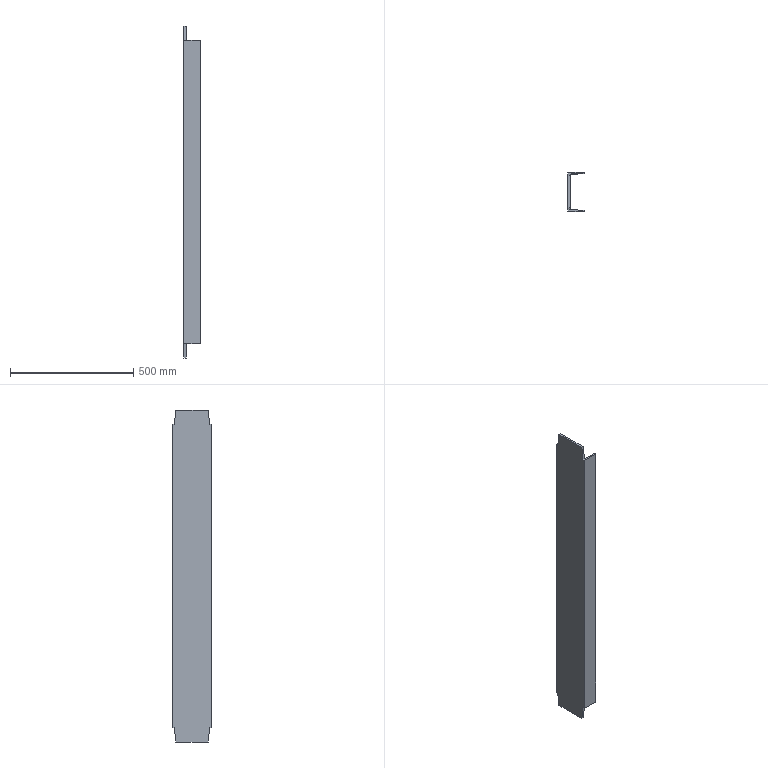Part | SolidWorks | features Extrusion 1, ICE 1 | 1 solid | 18 faces | box 65 x 160 x 1348 mm | volume 2648614 mm3 | plane 18
STEP:
#1=CARTESIAN_POINT('',(0.,146.,-674.));
#2=VERTEX_POINT('',#1);
#3=CARTESIAN_POINT('',(0.,14.,-674.));
#4=VERTEX_POINT('',#3);
#5=CARTESIAN_POINT('',(0.,0.,-674.));
#6=DIRECTION('',(0.,-1.,0.));
#7=VECTOR('',#6,1000.);
#8=LINE('',#5,#7);
#9=EDGE_CURVE('',#2,#4,#8,.T.);
#10=ORIENTED_EDGE('',*,*,#9,.T.);
#11=CARTESIAN_POINT('',(0.,8.,-617.));
#12=VERTEX_POINT('',#11);
#13=CARTESIAN_POINT('',(0.,8.,-617.));
#14=DIRECTION('',(0.,0.1047,-0.9945));
#15=VECTOR('',#14,1000.);
#16=LINE('',#13,#15);
#17=EDGE_CURVE('',#12,#4,#16,.T.);
#18=ORIENTED_EDGE('',*,*,#17,.F.);
#19=CARTESIAN_POINT('',(0.,0.,-617.));
#20=VERTEX_POINT('',#19);
#21=CARTESIAN_POINT('',(0.,0.,-617.));
#22=DIRECTION('',(0.,1.,0.));
#23=VECTOR('',#22,1000.);
#24=LINE('',#21,#23);
#25=EDGE_CURVE('',#20,#12,#24,.T.);
#26=ORIENTED_EDGE('',*,*,#25,.F.);
#27=CARTESIAN_POINT('',(0.,0.,617.));
#28=VERTEX_POINT('',#27);
#29=CARTESIAN_POINT('',(0.,0.,674.));
#30=DIRECTION('',(0.,0.,-1.));
#31=VECTOR('',#30,1000.);
#32=LINE('',#29,#31);
#33=EDGE_CURVE('',#28,#20,#32,.T.);
#34=ORIENTED_EDGE('',*,*,#33,.F.);
#35=CARTESIAN_POINT('',(0.,8.,617.));
#36=VERTEX_POINT('',#35);
#37=CARTESIAN_POINT('',(0.,0.,617.));
#38=DIRECTION('',(0.,-1.,0.));
#39=VECTOR('',#38,1000.);
#40=LINE('',#37,#39);
#41=EDGE_CURVE('',#36,#28,#40,.T.);
#42=ORIENTED_EDGE('',*,*,#41,.F.);
#43=CARTESIAN_POINT('',(0.,14.,674.));
#44=VERTEX_POINT('',#43);
#45=CARTESIAN_POINT('',(0.,8.,617.));
#46=DIRECTION('',(0.,-0.1047,-0.9945));
#47=VECTOR('',#46,1000.);
#48=LINE('',#45,#47);
#49=EDGE_CURVE('',#44,#36,#48,.T.);
#50=ORIENTED_EDGE('',*,*,#49,.F.);
#51=CARTESIAN_POINT('',(0.,146.,674.));
#52=VERTEX_POINT('',#51);
#53=CARTESIAN_POINT('',(0.,0.,674.));
#54=DIRECTION('',(0.,-1.,0.));
#55=VECTOR('',#54,1000.);
#56=LINE('',#53,#55);
#57=EDGE_CURVE('',#52,#44,#56,.T.);
#58=ORIENTED_EDGE('',*,*,#57,.F.);
#59=CARTESIAN_POINT('',(0.,152.,617.));
#60=VERTEX_POINT('',#59);
#61=CARTESIAN_POINT('',(0.,152.,617.));
#62=DIRECTION('',(0.,-0.1047,0.9945));
#63=VECTOR('',#62,1000.);
#64=LINE('',#61,#63);
#65=EDGE_CURVE('',#60,#52,#64,.T.);
#66=ORIENTED_EDGE('',*,*,#65,.F.);
#67=CARTESIAN_POINT('',(0.,160.,617.));
#68=VERTEX_POINT('',#67);
#69=CARTESIAN_POINT('',(0.,160.,617.));
#70=DIRECTION('',(0.,-1.,0.));
#71=VECTOR('',#70,1000.);
#72=LINE('',#69,#71);
#73=EDGE_CURVE('',#68,#60,#72,.T.);
#74=ORIENTED_EDGE('',*,*,#73,.F.);
#75=CARTESIAN_POINT('',(0.,160.,-617.));
#76=VERTEX_POINT('',#75);
#77=CARTESIAN_POINT('',(0.,160.,674.));
#78=DIRECTION('',(0.,0.,-1.));
#79=VECTOR('',#78,1000.);
#80=LINE('',#77,#79);
#81=EDGE_CURVE('',#68,#76,#80,.T.);
#82=ORIENTED_EDGE('',*,*,#81,.T.);
#83=CARTESIAN_POINT('',(0.,152.,-617.));
#84=VERTEX_POINT('',#83);
#85=CARTESIAN_POINT('',(0.,160.,-617.));
#86=DIRECTION('',(0.,1.,0.));
#87=VECTOR('',#86,1000.);
#88=LINE('',#85,#87);
#89=EDGE_CURVE('',#84,#76,#88,.T.);
#90=ORIENTED_EDGE('',*,*,#89,.F.);
#91=CARTESIAN_POINT('',(0.,152.,-617.));
#92=DIRECTION('',(0.,0.1047,0.9945));
#93=VECTOR('',#92,1000.);
#94=LINE('',#91,#93);
#95=EDGE_CURVE('',#2,#84,#94,.T.);
#96=ORIENTED_EDGE('',*,*,#95,.F.);
#97=EDGE_LOOP('',(#10,#18,#26,#34,#42,#50,#58,#66,#74,#82,#90,#96));
#98=FACE_OUTER_BOUND('',#97,.T.);
#99=CARTESIAN_POINT('',(0.,0.,674.));
#100=DIRECTION('',(1.,0.,0.));
#101=DIRECTION('',(0.,0.,-1.));
#102=AXIS2_PLACEMENT_3D('',#99,#100,#101);
#103=PLANE('',#102);
#104=ADVANCED_FACE('',(#98),#103,.F.);
#105=ORIENTED_EDGE('',*,*,#33,.T.);
#106=CARTESIAN_POINT('',(65.,0.,-617.));
#107=VERTEX_POINT('',#106);
#108=CARTESIAN_POINT('',(65.,0.,-617.));
#109=DIRECTION('',(-1.,0.,0.));
#110=VECTOR('',#109,1000.);
#111=LINE('',#108,#110);
#112=EDGE_CURVE('',#107,#20,#111,.T.);
#113=ORIENTED_EDGE('',*,*,#112,.F.);
#114=CARTESIAN_POINT('',(65.,0.,617.));
#115=VERTEX_POINT('',#114);
#116=CARTESIAN_POINT('',(65.,0.,674.));
#117=DIRECTION('',(0.,0.,-1.));
#118=VECTOR('',#117,1000.);
#119=LINE('',#116,#118);
#120=EDGE_CURVE('',#115,#107,#119,.T.);
#121=ORIENTED_EDGE('',*,*,#120,.F.);
#122=CARTESIAN_POINT('',(65.,0.,617.));
#123=DIRECTION('',(-1.,0.,0.));
#124=VECTOR('',#123,1000.);
#125=LINE('',#122,#124);
#126=EDGE_CURVE('',#115,#28,#125,.T.);
#127=ORIENTED_EDGE('',*,*,#126,.T.);
#128=EDGE_LOOP('',(#105,#113,#121,#127));
#129=FACE_OUTER_BOUND('',#128,.T.);
#130=CARTESIAN_POINT('',(0.,0.,674.));
#131=DIRECTION('',(0.,1.,0.));
#132=DIRECTION('',(0.,0.,1.));
#133=AXIS2_PLACEMENT_3D('',#130,#131,#132);
#134=PLANE('',#133);
#135=ADVANCED_FACE('',(#129),#134,.F.);
#136=ORIENTED_EDGE('',*,*,#120,.T.);
#137=CARTESIAN_POINT('',(65.,4.,-617.));
#138=VERTEX_POINT('',#137);
#139=CARTESIAN_POINT('',(65.,0.,-617.));
#140=DIRECTION('',(0.,1.,0.));
#141=VECTOR('',#140,1000.);
#142=LINE('',#139,#141);
#143=EDGE_CURVE('',#107,#138,#142,.T.);
#144=ORIENTED_EDGE('',*,*,#143,.T.);
#145=CARTESIAN_POINT('',(65.,4.,617.));
#146=VERTEX_POINT('',#145);
#147=CARTESIAN_POINT('',(65.,4.,674.));
#148=DIRECTION('',(0.,0.,-1.));
#149=VECTOR('',#148,1000.);
#150=LINE('',#147,#149);
#151=EDGE_CURVE('',#146,#138,#150,.T.);
#152=ORIENTED_EDGE('',*,*,#151,.F.);
#153=CARTESIAN_POINT('',(65.,0.,617.));
#154=DIRECTION('',(0.,-1.,0.));
#155=VECTOR('',#154,1000.);
#156=LINE('',#153,#155);
#157=EDGE_CURVE('',#146,#115,#156,.T.);
#158=ORIENTED_EDGE('',*,*,#157,.T.);
#159=EDGE_LOOP('',(#136,#144,#152,#158));
#160=FACE_OUTER_BOUND('',#159,.T.);
#161=CARTESIAN_POINT('',(65.,0.,674.));
#162=DIRECTION('',(-1.,0.,0.));
#163=DIRECTION('',(0.,0.,1.));
#164=AXIS2_PLACEMENT_3D('',#161,#162,#163);
#165=PLANE('',#164);
#166=ADVANCED_FACE('',(#160),#165,.F.);
#167=ORIENTED_EDGE('',*,*,#151,.T.);
#168=CARTESIAN_POINT('',(8.5,8.,-617.));
#169=VERTEX_POINT('',#168);
#170=CARTESIAN_POINT('',(65.,4.,-617.));
#171=DIRECTION('',(-0.9975,0.07062,0.));
#172=VECTOR('',#171,1000.);
#173=LINE('',#170,#172);
#174=EDGE_CURVE('',#138,#169,#173,.T.);
#175=ORIENTED_EDGE('',*,*,#174,.T.);
#176=CARTESIAN_POINT('',(8.5,8.,617.));
#177=VERTEX_POINT('',#176);
#178=CARTESIAN_POINT('',(8.5,8.,674.));
#179=DIRECTION('',(0.,0.,-1.));
#180=VECTOR('',#179,1000.);
#181=LINE('',#178,#180);
#182=EDGE_CURVE('',#177,#169,#181,.T.);
#183=ORIENTED_EDGE('',*,*,#182,.F.);
#184=CARTESIAN_POINT('',(65.,4.,617.));
#185=DIRECTION('',(0.9975,-0.07062,0.));
#186=VECTOR('',#185,1000.);
#187=LINE('',#184,#186);
#188=EDGE_CURVE('',#177,#146,#187,.T.);
#189=ORIENTED_EDGE('',*,*,#188,.T.);
#190=EDGE_LOOP('',(#167,#175,#183,#189));
#191=FACE_OUTER_BOUND('',#190,.T.);
#192=CARTESIAN_POINT('',(65.,4.,674.));
#193=DIRECTION('',(-0.07062,-0.9975,0.));
#194=DIRECTION('',(0.9975,-0.07062,0.));
#195=AXIS2_PLACEMENT_3D('',#192,#193,#194);
#196=PLANE('',#195);
#197=ADVANCED_FACE('',(#191),#196,.F.);
#198=ORIENTED_EDGE('',*,*,#182,.T.);
#199=CARTESIAN_POINT('',(8.5,14.,-674.));
#200=VERTEX_POINT('',#199);
#201=CARTESIAN_POINT('',(8.5,-126.405,659.852));
#202=DIRECTION('',(0.,0.1047,-0.9945));
#203=VECTOR('',#202,1000.);
#204=LINE('',#201,#203);
#205=EDGE_CURVE('',#169,#200,#204,.T.);
#206=ORIENTED_EDGE('',*,*,#205,.T.);
#207=CARTESIAN_POINT('',(8.5,146.,-674.));
#208=VERTEX_POINT('',#207);
#209=CARTESIAN_POINT('',(8.5,8.,-674.));
#210=DIRECTION('',(0.,1.,0.));
#211=VECTOR('',#210,1000.);
#212=LINE('',#209,#211);
#213=EDGE_CURVE('',#200,#208,#212,.T.);
#214=ORIENTED_EDGE('',*,*,#213,.T.);
#215=CARTESIAN_POINT('',(8.5,152.,-617.));
#216=VERTEX_POINT('',#215);
#217=CARTESIAN_POINT('',(8.5,284.827,644.86));
#218=DIRECTION('',(0.,0.1047,0.9945));
#219=VECTOR('',#218,1000.);
#220=LINE('',#217,#219);
#221=EDGE_CURVE('',#208,#216,#220,.T.);
#222=ORIENTED_EDGE('',*,*,#221,.T.);
#223=CARTESIAN_POINT('',(8.5,152.,617.));
#224=VERTEX_POINT('',#223);
#225=CARTESIAN_POINT('',(8.5,152.,674.));
#226=DIRECTION('',(0.,0.,-1.));
#227=VECTOR('',#226,1000.);
#228=LINE('',#225,#227);
#229=EDGE_CURVE('',#224,#216,#228,.T.);
#230=ORIENTED_EDGE('',*,*,#229,.F.);
#231=CARTESIAN_POINT('',(8.5,146.,674.));
#232=VERTEX_POINT('',#231);
#233=CARTESIAN_POINT('',(8.5,144.488,688.367));
#234=DIRECTION('',(0.,-0.1047,0.9945));
#235=VECTOR('',#234,1000.);
#236=LINE('',#233,#235);
#237=EDGE_CURVE('',#224,#232,#236,.T.);
#238=ORIENTED_EDGE('',*,*,#237,.T.);
#239=CARTESIAN_POINT('',(8.5,14.,674.));
#240=VERTEX_POINT('',#239);
#241=CARTESIAN_POINT('',(8.5,8.,674.));
#242=DIRECTION('',(0.,1.,0.));
#243=VECTOR('',#242,1000.);
#244=LINE('',#241,#243);
#245=EDGE_CURVE('',#240,#232,#244,.T.);
#246=ORIENTED_EDGE('',*,*,#245,.F.);
#247=CARTESIAN_POINT('',(8.5,13.934,673.375));
#248=DIRECTION('',(0.,-0.1047,-0.9945));
#249=VECTOR('',#248,1000.);
#250=LINE('',#247,#249);
#251=EDGE_CURVE('',#240,#177,#250,.T.);
#252=ORIENTED_EDGE('',*,*,#251,.T.);
#253=EDGE_LOOP('',(#198,#206,#214,#222,#230,#238,#246,#252));
#254=FACE_OUTER_BOUND('',#253,.T.);
#255=CARTESIAN_POINT('',(8.5,8.,674.));
#256=DIRECTION('',(-1.,0.,0.));
#257=DIRECTION('',(0.,0.,1.));
#258=AXIS2_PLACEMENT_3D('',#255,#256,#257);
#259=PLANE('',#258);
#260=ADVANCED_FACE('',(#254),#259,.F.);
#261=CARTESIAN_POINT('',(65.,156.,617.));
#262=VERTEX_POINT('',#261);
#263=CARTESIAN_POINT('',(65.,156.,-617.));
#264=VERTEX_POINT('',#263);
#265=CARTESIAN_POINT('',(65.,156.,674.));
#266=DIRECTION('',(0.,0.,-1.));
#267=VECTOR('',#266,1000.);
#268=LINE('',#265,#267);
#269=EDGE_CURVE('',#262,#264,#268,.T.);
#270=ORIENTED_EDGE('',*,*,#269,.F.);
#271=CARTESIAN_POINT('',(65.,156.,617.));
#272=DIRECTION('',(-0.9975,-0.07062,0.));
#273=VECTOR('',#272,1000.);
#274=LINE('',#271,#273);
#275=EDGE_CURVE('',#262,#224,#274,.T.);
#276=ORIENTED_EDGE('',*,*,#275,.T.);
#277=ORIENTED_EDGE('',*,*,#229,.T.);
#278=CARTESIAN_POINT('',(65.,156.,-617.));
#279=DIRECTION('',(0.9975,0.07062,0.));
#280=VECTOR('',#279,1000.);
#281=LINE('',#278,#280);
#282=EDGE_CURVE('',#216,#264,#281,.T.);
#283=ORIENTED_EDGE('',*,*,#282,.T.);
#284=EDGE_LOOP('',(#270,#276,#277,#283));
#285=FACE_OUTER_BOUND('',#284,.T.);
#286=CARTESIAN_POINT('',(65.,156.,674.));
#287=DIRECTION('',(-0.07062,0.9975,0.));
#288=DIRECTION('',(-0.9975,-0.07062,0.));
#289=AXIS2_PLACEMENT_3D('',#286,#287,#288);
#290=PLANE('',#289);
#291=ADVANCED_FACE('',(#285),#290,.F.);
#292=CARTESIAN_POINT('',(65.,160.,617.));
#293=VERTEX_POINT('',#292);
#294=CARTESIAN_POINT('',(65.,160.,-617.));
#295=VERTEX_POINT('',#294);
#296=CARTESIAN_POINT('',(65.,160.,674.));
#297=DIRECTION('',(0.,0.,-1.));
#298=VECTOR('',#297,1000.);
#299=LINE('',#296,#298);
#300=EDGE_CURVE('',#293,#295,#299,.T.);
#301=ORIENTED_EDGE('',*,*,#300,.F.);
#302=CARTESIAN_POINT('',(65.,160.,617.));
#303=DIRECTION('',(0.,-1.,0.));
#304=VECTOR('',#303,1000.);
#305=LINE('',#302,#304);
#306=EDGE_CURVE('',#293,#262,#305,.T.);
#307=ORIENTED_EDGE('',*,*,#306,.T.);
#308=ORIENTED_EDGE('',*,*,#269,.T.);
#309=CARTESIAN_POINT('',(65.,160.,-617.));
#310=DIRECTION('',(0.,1.,0.));
#311=VECTOR('',#310,1000.);
#312=LINE('',#309,#311);
#313=EDGE_CURVE('',#264,#295,#312,.T.);
#314=ORIENTED_EDGE('',*,*,#313,.T.);
#315=EDGE_LOOP('',(#301,#307,#308,#314));
#316=FACE_OUTER_BOUND('',#315,.T.);
#317=CARTESIAN_POINT('',(65.,160.,674.));
#318=DIRECTION('',(-1.,0.,0.));
#319=DIRECTION('',(0.,0.,1.));
#320=AXIS2_PLACEMENT_3D('',#317,#318,#319);
#321=PLANE('',#320);
#322=ADVANCED_FACE('',(#316),#321,.F.);
#323=ORIENTED_EDGE('',*,*,#81,.F.);
#324=CARTESIAN_POINT('',(65.,160.,617.));
#325=DIRECTION('',(-1.,0.,0.));
#326=VECTOR('',#325,1000.);
#327=LINE('',#324,#326);
#328=EDGE_CURVE('',#293,#68,#327,.T.);
#329=ORIENTED_EDGE('',*,*,#328,.F.);
#330=ORIENTED_EDGE('',*,*,#300,.T.);
#331=CARTESIAN_POINT('',(65.,160.,-617.));
#332=DIRECTION('',(-1.,0.,0.));
#333=VECTOR('',#332,1000.);
#334=LINE('',#331,#333);
#335=EDGE_CURVE('',#295,#76,#334,.T.);
#336=ORIENTED_EDGE('',*,*,#335,.T.);
#337=EDGE_LOOP('',(#323,#329,#330,#336));
#338=FACE_OUTER_BOUND('',#337,.T.);
#339=CARTESIAN_POINT('',(0.,160.,674.));
#340=DIRECTION('',(0.,-1.,0.));
#341=DIRECTION('',(1.,0.,0.));
#342=AXIS2_PLACEMENT_3D('',#339,#340,#341);
#343=PLANE('',#342);
#344=ADVANCED_FACE('',(#338),#343,.F.);
#345=ORIENTED_EDGE('',*,*,#57,.T.);
#346=CARTESIAN_POINT('',(0.,14.,674.));
#347=DIRECTION('',(1.,0.,0.));
#348=VECTOR('',#347,1000.);
#349=LINE('',#346,#348);
#350=EDGE_CURVE('',#44,#240,#349,.T.);
#351=ORIENTED_EDGE('',*,*,#350,.T.);
#352=ORIENTED_EDGE('',*,*,#245,.T.);
#353=CARTESIAN_POINT('',(0.,146.,674.));
#354=DIRECTION('',(-1.,0.,0.));
#355=VECTOR('',#354,1000.);
#356=LINE('',#353,#355);
#357=EDGE_CURVE('',#232,#52,#356,.T.);
#358=ORIENTED_EDGE('',*,*,#357,.T.);
#359=EDGE_LOOP('',(#345,#351,#352,#358));
#360=FACE_OUTER_BOUND('',#359,.T.);
#361=CARTESIAN_POINT('',(0.,0.,674.));
#362=DIRECTION('',(0.,0.,-1.));
#363=DIRECTION('',(-1.,0.,0.));
#364=AXIS2_PLACEMENT_3D('',#361,#362,#363);
#365=PLANE('',#364);
#366=ADVANCED_FACE('',(#360),#365,.F.);
#367=CARTESIAN_POINT('',(0.,14.,-674.));
#368=DIRECTION('',(1.,0.,0.));
#369=VECTOR('',#368,1000.);
#370=LINE('',#367,#369);
#371=EDGE_CURVE('',#4,#200,#370,.T.);
#372=ORIENTED_EDGE('',*,*,#371,.F.);
#373=ORIENTED_EDGE('',*,*,#9,.F.);
#374=CARTESIAN_POINT('',(0.,146.,-674.));
#375=DIRECTION('',(-1.,0.,0.));
#376=VECTOR('',#375,1000.);
#377=LINE('',#374,#376);
#378=EDGE_CURVE('',#208,#2,#377,.T.);
#379=ORIENTED_EDGE('',*,*,#378,.F.);
#380=ORIENTED_EDGE('',*,*,#213,.F.);
#381=EDGE_LOOP('',(#372,#373,#379,#380));
#382=FACE_OUTER_BOUND('',#381,.T.);
#383=CARTESIAN_POINT('',(0.,0.,-674.));
#384=DIRECTION('',(0.,0.,-1.));
#385=DIRECTION('',(-1.,0.,0.));
#386=AXIS2_PLACEMENT_3D('',#383,#384,#385);
#387=PLANE('',#386);
#388=ADVANCED_FACE('',(#382),#387,.T.);
#389=CARTESIAN_POINT('',(65.,152.,-617.));
#390=DIRECTION('',(-1.,0.,0.));
#391=VECTOR('',#390,1000.);
#392=LINE('',#389,#391);
#393=EDGE_CURVE('',#216,#84,#392,.T.);
#394=ORIENTED_EDGE('',*,*,#393,.T.);
#395=ORIENTED_EDGE('',*,*,#89,.T.);
#396=ORIENTED_EDGE('',*,*,#335,.F.);
#397=ORIENTED_EDGE('',*,*,#313,.F.);
#398=ORIENTED_EDGE('',*,*,#282,.F.);
#399=EDGE_LOOP('',(#394,#395,#396,#397,#398));
#400=FACE_OUTER_BOUND('',#399,.T.);
#401=CARTESIAN_POINT('',(65.,160.,-617.));
#402=DIRECTION('',(0.,0.,1.));
#403=DIRECTION('',(0.,-1.,0.));
#404=AXIS2_PLACEMENT_3D('',#401,#402,#403);
#405=PLANE('',#404);
#406=ADVANCED_FACE('',(#400),#405,.F.);
#407=ORIENTED_EDGE('',*,*,#378,.T.);
#408=ORIENTED_EDGE('',*,*,#95,.T.);
#409=ORIENTED_EDGE('',*,*,#393,.F.);
#410=ORIENTED_EDGE('',*,*,#221,.F.);
#411=EDGE_LOOP('',(#407,#408,#409,#410));
#412=FACE_OUTER_BOUND('',#411,.T.);
#413=CARTESIAN_POINT('',(65.,152.,-617.));
#414=DIRECTION('',(0.,-0.9945,0.1047));
#415=DIRECTION('',(0.,-0.1047,-0.9945));
#416=AXIS2_PLACEMENT_3D('',#413,#414,#415);
#417=PLANE('',#416);
#418=ADVANCED_FACE('',(#412),#417,.F.);
#419=ORIENTED_EDGE('',*,*,#143,.F.);
#420=ORIENTED_EDGE('',*,*,#112,.T.);
#421=ORIENTED_EDGE('',*,*,#25,.T.);
#422=CARTESIAN_POINT('',(65.,8.,-617.));
#423=DIRECTION('',(-1.,0.,0.));
#424=VECTOR('',#423,1000.);
#425=LINE('',#422,#424);
#426=EDGE_CURVE('',#169,#12,#425,.T.);
#427=ORIENTED_EDGE('',*,*,#426,.F.);
#428=ORIENTED_EDGE('',*,*,#174,.F.);
#429=EDGE_LOOP('',(#419,#420,#421,#427,#428));
#430=FACE_OUTER_BOUND('',#429,.T.);
#431=CARTESIAN_POINT('',(65.,0.,-617.));
#432=DIRECTION('',(0.,0.,1.));
#433=DIRECTION('',(0.,-1.,0.));
#434=AXIS2_PLACEMENT_3D('',#431,#432,#433);
#435=PLANE('',#434);
#436=ADVANCED_FACE('',(#430),#435,.F.);
#437=ORIENTED_EDGE('',*,*,#426,.T.);
#438=ORIENTED_EDGE('',*,*,#17,.T.);
#439=ORIENTED_EDGE('',*,*,#371,.T.);
#440=ORIENTED_EDGE('',*,*,#205,.F.);
#441=EDGE_LOOP('',(#437,#438,#439,#440));
#442=FACE_OUTER_BOUND('',#441,.T.);
#443=CARTESIAN_POINT('',(65.,8.,-617.));
#444=DIRECTION('',(0.,0.9945,0.1047));
#445=DIRECTION('',(0.,-0.1047,0.9945));
#446=AXIS2_PLACEMENT_3D('',#443,#444,#445);
#447=PLANE('',#446);
#448=ADVANCED_FACE('',(#442),#447,.F.);
#449=ORIENTED_EDGE('',*,*,#306,.F.);
#450=ORIENTED_EDGE('',*,*,#328,.T.);
#451=ORIENTED_EDGE('',*,*,#73,.T.);
#452=CARTESIAN_POINT('',(65.,152.,617.));
#453=DIRECTION('',(-1.,0.,0.));
#454=VECTOR('',#453,1000.);
#455=LINE('',#452,#454);
#456=EDGE_CURVE('',#224,#60,#455,.T.);
#457=ORIENTED_EDGE('',*,*,#456,.F.);
#458=ORIENTED_EDGE('',*,*,#275,.F.);
#459=EDGE_LOOP('',(#449,#450,#451,#457,#458));
#460=FACE_OUTER_BOUND('',#459,.T.);
#461=CARTESIAN_POINT('',(65.,160.,617.));
#462=DIRECTION('',(0.,0.,-1.));
#463=DIRECTION('',(0.,1.,0.));
#464=AXIS2_PLACEMENT_3D('',#461,#462,#463);
#465=PLANE('',#464);
#466=ADVANCED_FACE('',(#460),#465,.F.);
#467=ORIENTED_EDGE('',*,*,#456,.T.);
#468=ORIENTED_EDGE('',*,*,#65,.T.);
#469=ORIENTED_EDGE('',*,*,#357,.F.);
#470=ORIENTED_EDGE('',*,*,#237,.F.);
#471=EDGE_LOOP('',(#467,#468,#469,#470));
#472=FACE_OUTER_BOUND('',#471,.T.);
#473=CARTESIAN_POINT('',(65.,152.,617.));
#474=DIRECTION('',(0.,-0.9945,-0.1047));
#475=DIRECTION('',(0.,0.1047,-0.9945));
#476=AXIS2_PLACEMENT_3D('',#473,#474,#475);
#477=PLANE('',#476);
#478=ADVANCED_FACE('',(#472),#477,.F.);
#479=CARTESIAN_POINT('',(65.,8.,617.));
#480=DIRECTION('',(-1.,0.,0.));
#481=VECTOR('',#480,1000.);
#482=LINE('',#479,#481);
#483=EDGE_CURVE('',#177,#36,#482,.T.);
#484=ORIENTED_EDGE('',*,*,#483,.T.);
#485=ORIENTED_EDGE('',*,*,#41,.T.);
#486=ORIENTED_EDGE('',*,*,#126,.F.);
#487=ORIENTED_EDGE('',*,*,#157,.F.);
#488=ORIENTED_EDGE('',*,*,#188,.F.);
#489=EDGE_LOOP('',(#484,#485,#486,#487,#488));
#490=FACE_OUTER_BOUND('',#489,.T.);
#491=CARTESIAN_POINT('',(65.,0.,617.));
#492=DIRECTION('',(0.,0.,-1.));
#493=DIRECTION('',(0.,1.,0.));
#494=AXIS2_PLACEMENT_3D('',#491,#492,#493);
#495=PLANE('',#494);
#496=ADVANCED_FACE('',(#490),#495,.F.);
#497=ORIENTED_EDGE('',*,*,#350,.F.);
#498=ORIENTED_EDGE('',*,*,#49,.T.);
#499=ORIENTED_EDGE('',*,*,#483,.F.);
#500=ORIENTED_EDGE('',*,*,#251,.F.);
#501=EDGE_LOOP('',(#497,#498,#499,#500));
#502=FACE_OUTER_BOUND('',#501,.T.);
#503=CARTESIAN_POINT('',(65.,8.,617.));
#504=DIRECTION('',(0.,0.9945,-0.1047));
#505=DIRECTION('',(0.,0.1047,0.9945));
#506=AXIS2_PLACEMENT_3D('',#503,#504,#505);
#507=PLANE('',#506);
#508=ADVANCED_FACE('',(#502),#507,.F.);
#509=CLOSED_SHELL('',(#104,#135,#166,#197,#260,#291,#322,#344,#366,#388,#406,#418,#436,#448,#466,#478,#496,#508));
#510=MANIFOLD_SOLID_BREP('',#509);
#511=CARTESIAN_POINT('',(0.,0.,0.));
#512=DIRECTION('',(0.,0.,1.));
#513=DIRECTION('',(1.,0.,0.));
#514=AXIS2_PLACEMENT_3D('',#511,#512,#513);
#515=(LENGTH_UNIT()NAMED_UNIT(*)SI_UNIT(.MILLI.,.METRE.));
#516=UNCERTAINTY_MEASURE_WITH_UNIT(LENGTH_MEASURE(0.00001),#515,'','');
#517=(NAMED_UNIT(*)PLANE_ANGLE_UNIT()SI_UNIT($,.RADIAN.));
#518=(NAMED_UNIT(*)SI_UNIT($,.STERADIAN.)SOLID_ANGLE_UNIT());
#519=(GEOMETRIC_REPRESENTATION_CONTEXT(3)GLOBAL_UNCERTAINTY_ASSIGNED_CONTEXT((#516))GLOBAL_UNIT_ASSIGNED_CONTEXT((#515,#517,#518))REPRESENTATION_CONTEXT('',''));
#520=ADVANCED_BREP_SHAPE_REPRESENTATION('',(#510,#514),#519);